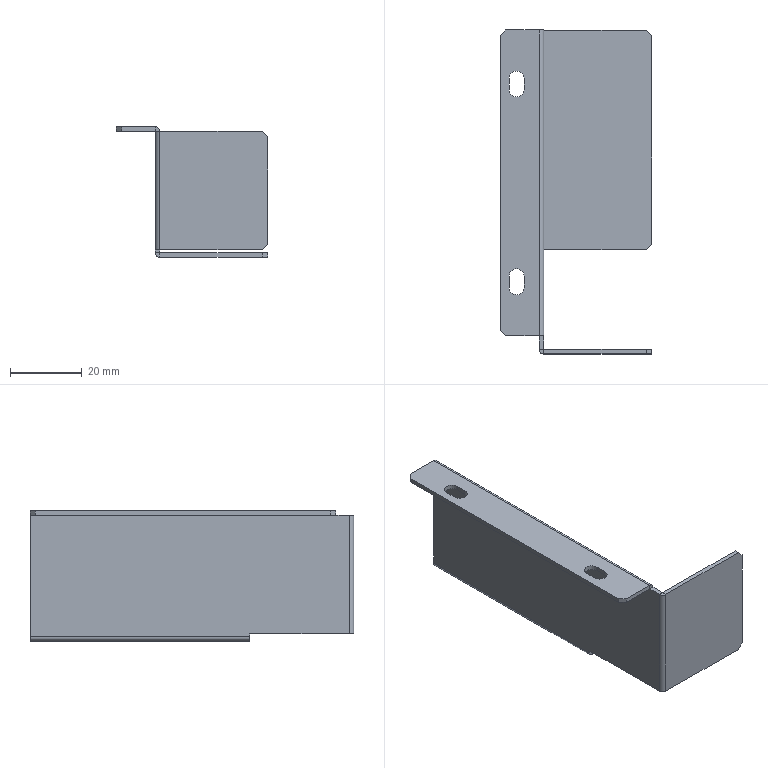Part | STEP file | 1 solid | 47 faces | box 42 x 90 x 36.2 mm | volume 8185 mm3 | plane 37 | cylinder 10 | commonest cylinder face diameters 4.2 x4 0.1 x3 2.5 x3